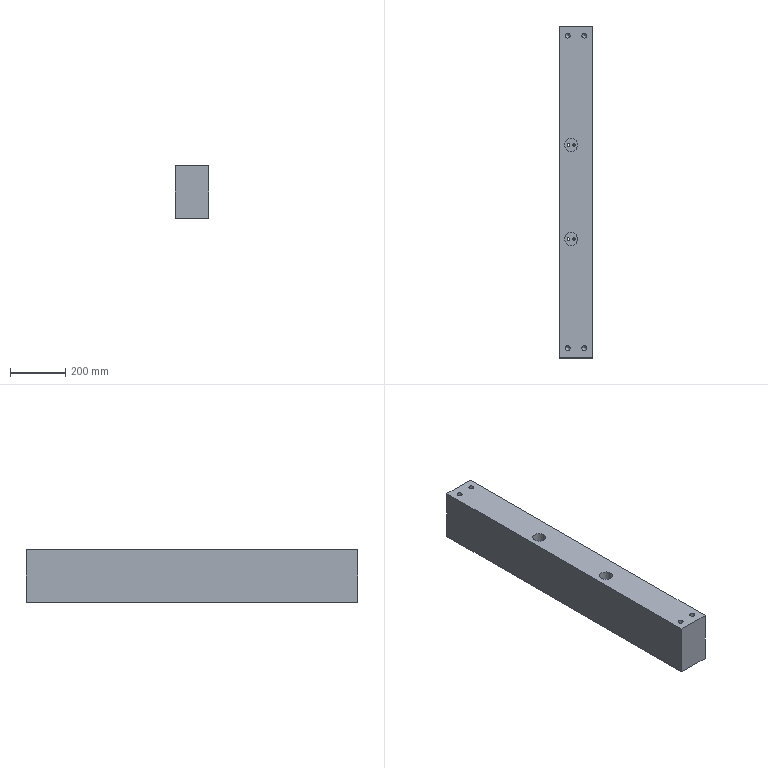Part | STEP file | lll_id4470_x_t | 1 solid | 38 faces | box 120 x 1200 x 190 mm | volume 26849134 mm3 | cylinder 18 | plane 12 | cone 8 | commonest cylinder face diameters 9 x4 14 x4 17.505 x4 17.506 x4 47 x2
STEP:
#1=CARTESIAN_POINT('',(1831.188,565.,-370.));
#2=VERTEX_POINT('',#1);
#3=CARTESIAN_POINT('',(1822.435,565.,-370.));
#4=DIRECTION('',(0.,0.,1.));
#5=DIRECTION('',(1.,0.,0.));
#6=AXIS2_PLACEMENT_3D('',#3,#4,#5);
#7=CIRCLE('',#6,8.752);
#8=EDGE_CURVE('',#2,#2,#7,.T.);
#9=ORIENTED_EDGE('',*,*,#8,.T.);
#10=EDGE_LOOP('',(#9));
#11=FACE_BOUND('',#10,.T.);
#12=CARTESIAN_POINT('',(1831.188,-565.,-370.));
#13=VERTEX_POINT('',#12);
#14=CARTESIAN_POINT('',(1822.435,-565.,-370.));
#15=DIRECTION('',(0.,0.,1.));
#16=DIRECTION('',(1.,0.,0.));
#17=AXIS2_PLACEMENT_3D('',#14,#15,#16);
#18=CIRCLE('',#17,8.752);
#19=EDGE_CURVE('',#13,#13,#18,.T.);
#20=ORIENTED_EDGE('',*,*,#19,.T.);
#21=EDGE_LOOP('',(#20));
#22=FACE_BOUND('',#21,.T.);
#23=CARTESIAN_POINT('',(1778.,-170.,-370.));
#24=VERTEX_POINT('',#23);
#25=CARTESIAN_POINT('',(1785.,-170.,-370.));
#26=DIRECTION('',(0.,0.,1.));
#27=DIRECTION('',(-1.,0.,0.));
#28=AXIS2_PLACEMENT_3D('',#25,#26,#27);
#29=CIRCLE('',#28,7.);
#30=EDGE_CURVE('',#24,#24,#29,.T.);
#31=ORIENTED_EDGE('',*,*,#30,.T.);
#32=EDGE_LOOP('',(#31));
#33=FACE_BOUND('',#32,.T.);
#34=CARTESIAN_POINT('',(1778.,170.,-370.));
#35=VERTEX_POINT('',#34);
#36=CARTESIAN_POINT('',(1785.,170.,-370.));
#37=DIRECTION('',(0.,0.,1.));
#38=DIRECTION('',(-1.,0.,0.));
#39=AXIS2_PLACEMENT_3D('',#36,#37,#38);
#40=CIRCLE('',#39,7.);
#41=EDGE_CURVE('',#35,#35,#40,.T.);
#42=ORIENTED_EDGE('',*,*,#41,.T.);
#43=EDGE_LOOP('',(#42));
#44=FACE_BOUND('',#43,.T.);
#45=CARTESIAN_POINT('',(1758.,170.,-370.));
#46=VERTEX_POINT('',#45);
#47=CARTESIAN_POINT('',(1765.,170.,-370.));
#48=DIRECTION('',(0.,0.,1.));
#49=DIRECTION('',(-1.,0.,0.));
#50=AXIS2_PLACEMENT_3D('',#47,#48,#49);
#51=CIRCLE('',#50,7.);
#52=EDGE_CURVE('',#46,#46,#51,.T.);
#53=ORIENTED_EDGE('',*,*,#52,.T.);
#54=EDGE_LOOP('',(#53));
#55=FACE_BOUND('',#54,.T.);
#56=CARTESIAN_POINT('',(1758.,-170.,-370.));
#57=VERTEX_POINT('',#56);
#58=CARTESIAN_POINT('',(1765.,-170.,-370.));
#59=DIRECTION('',(0.,0.,1.));
#60=DIRECTION('',(-1.,0.,0.));
#61=AXIS2_PLACEMENT_3D('',#58,#59,#60);
#62=CIRCLE('',#61,7.);
#63=EDGE_CURVE('',#57,#57,#62,.T.);
#64=ORIENTED_EDGE('',*,*,#63,.T.);
#65=EDGE_LOOP('',(#64));
#66=FACE_BOUND('',#65,.T.);
#67=CARTESIAN_POINT('',(1852.435,600.,-370.));
#68=VERTEX_POINT('',#67);
#69=CARTESIAN_POINT('',(1852.435,-600.,-370.));
#70=VERTEX_POINT('',#69);
#71=CARTESIAN_POINT('',(1852.435,600.,-370.));
#72=DIRECTION('',(0.,-1.,0.));
#73=VECTOR('',#72,1.);
#74=LINE('',#71,#73);
#75=EDGE_CURVE('',#68,#70,#74,.T.);
#76=ORIENTED_EDGE('',*,*,#75,.T.);
#77=CARTESIAN_POINT('',(1732.435,-600.,-370.));
#78=VERTEX_POINT('',#77);
#79=CARTESIAN_POINT('',(1852.435,-600.,-370.));
#80=DIRECTION('',(-1.,0.,0.));
#81=VECTOR('',#80,1.);
#82=LINE('',#79,#81);
#83=EDGE_CURVE('',#70,#78,#82,.T.);
#84=ORIENTED_EDGE('',*,*,#83,.T.);
#85=CARTESIAN_POINT('',(1732.435,600.,-370.));
#86=VERTEX_POINT('',#85);
#87=CARTESIAN_POINT('',(1732.435,1.,-370.));
#88=DIRECTION('',(0.,-1.,0.));
#89=VECTOR('',#88,1.);
#90=LINE('',#87,#89);
#91=EDGE_CURVE('',#86,#78,#90,.T.);
#92=ORIENTED_EDGE('',*,*,#91,.F.);
#93=CARTESIAN_POINT('',(-2117.565,600.,-370.));
#94=DIRECTION('',(1.,0.,0.));
#95=VECTOR('',#94,1.);
#96=LINE('',#93,#95);
#97=EDGE_CURVE('',#86,#68,#96,.T.);
#98=ORIENTED_EDGE('',*,*,#97,.T.);
#99=EDGE_LOOP('',(#76,#84,#92,#98));
#100=FACE_BOUND('',#99,.T.);
#101=CARTESIAN_POINT('',(1771.188,565.,-370.));
#102=VERTEX_POINT('',#101);
#103=CARTESIAN_POINT('',(1762.435,565.,-370.));
#104=DIRECTION('',(0.,0.,1.));
#105=DIRECTION('',(1.,0.,0.));
#106=AXIS2_PLACEMENT_3D('',#103,#104,#105);
#107=CIRCLE('',#106,8.752);
#108=EDGE_CURVE('',#102,#102,#107,.T.);
#109=ORIENTED_EDGE('',*,*,#108,.T.);
#110=EDGE_LOOP('',(#109));
#111=FACE_BOUND('',#110,.T.);
#112=CARTESIAN_POINT('',(1771.188,-565.,-370.));
#113=VERTEX_POINT('',#112);
#114=CARTESIAN_POINT('',(1762.435,-565.,-370.));
#115=DIRECTION('',(0.,0.,1.));
#116=DIRECTION('',(1.,0.,0.));
#117=AXIS2_PLACEMENT_3D('',#114,#115,#116);
#118=CIRCLE('',#117,8.752);
#119=EDGE_CURVE('',#113,#113,#118,.T.);
#120=ORIENTED_EDGE('',*,*,#119,.T.);
#121=EDGE_LOOP('',(#120));
#122=FACE_BOUND('',#121,.T.);
#123=CARTESIAN_POINT('',(4038.751,1.,-370.));
#124=DIRECTION('',(0.,0.,-1.));
#125=DIRECTION('',(-1.,0.,0.));
#126=AXIS2_PLACEMENT_3D('',#123,#124,#125);
#127=PLANE('',#126);
#128=ADVANCED_FACE('',(#11,#22,#33,#44,#55,#66,#100,#111,#122),#127,.T.);
#129=CARTESIAN_POINT('',(1852.435,600.,-180.));
#130=VERTEX_POINT('',#129);
#131=CARTESIAN_POINT('',(1852.435,-600.,-180.));
#132=VERTEX_POINT('',#131);
#133=CARTESIAN_POINT('',(1852.435,1.,-180.));
#134=DIRECTION('',(0.,-1.,0.));
#135=VECTOR('',#134,1.);
#136=LINE('',#133,#135);
#137=EDGE_CURVE('',#130,#132,#136,.T.);
#138=ORIENTED_EDGE('',*,*,#137,.T.);
#139=CARTESIAN_POINT('',(1852.435,-600.,-182.5));
#140=DIRECTION('',(0.,0.,-1.));
#141=VECTOR('',#140,1.);
#142=LINE('',#139,#141);
#143=EDGE_CURVE('',#132,#70,#142,.T.);
#144=ORIENTED_EDGE('',*,*,#143,.T.);
#145=ORIENTED_EDGE('',*,*,#75,.F.);
#146=CARTESIAN_POINT('',(1852.435,600.,-182.5));
#147=DIRECTION('',(0.,0.,-1.));
#148=VECTOR('',#147,1.);
#149=LINE('',#146,#148);
#150=EDGE_CURVE('',#130,#68,#149,.T.);
#151=ORIENTED_EDGE('',*,*,#150,.F.);
#152=EDGE_LOOP('',(#138,#144,#145,#151));
#153=FACE_OUTER_BOUND('',#152,.T.);
#154=CARTESIAN_POINT('',(1852.435,600.,-182.5));
#155=DIRECTION('',(1.,0.,0.));
#156=DIRECTION('',(0.,0.,-1.));
#157=AXIS2_PLACEMENT_3D('',#154,#155,#156);
#158=PLANE('',#157);
#159=ADVANCED_FACE('',(#153),#158,.T.);
#160=CARTESIAN_POINT('',(1753.682,565.,-180.));
#161=VERTEX_POINT('',#160);
#162=CARTESIAN_POINT('',(1762.435,565.,-180.));
#163=DIRECTION('',(0.,0.,-1.));
#164=DIRECTION('',(-1.,0.,0.));
#165=AXIS2_PLACEMENT_3D('',#162,#163,#164);
#166=CIRCLE('',#165,8.753);
#167=EDGE_CURVE('',#161,#161,#166,.T.);
#168=ORIENTED_EDGE('',*,*,#167,.T.);
#169=EDGE_LOOP('',(#168));
#170=FACE_BOUND('',#169,.T.);
#171=CARTESIAN_POINT('',(1753.682,-565.,-180.));
#172=VERTEX_POINT('',#171);
#173=CARTESIAN_POINT('',(1762.435,-565.,-180.));
#174=DIRECTION('',(0.,0.,-1.));
#175=DIRECTION('',(-1.,0.,0.));
#176=AXIS2_PLACEMENT_3D('',#173,#174,#175);
#177=CIRCLE('',#176,8.753);
#178=EDGE_CURVE('',#172,#172,#177,.T.);
#179=ORIENTED_EDGE('',*,*,#178,.T.);
#180=EDGE_LOOP('',(#179));
#181=FACE_BOUND('',#180,.T.);
#182=CARTESIAN_POINT('',(1813.682,-565.,-180.));
#183=VERTEX_POINT('',#182);
#184=CARTESIAN_POINT('',(1822.435,-565.,-180.));
#185=DIRECTION('',(0.,0.,-1.));
#186=DIRECTION('',(-1.,0.,0.));
#187=AXIS2_PLACEMENT_3D('',#184,#185,#186);
#188=CIRCLE('',#187,8.753);
#189=EDGE_CURVE('',#183,#183,#188,.T.);
#190=ORIENTED_EDGE('',*,*,#189,.T.);
#191=EDGE_LOOP('',(#190));
#192=FACE_BOUND('',#191,.T.);
#193=CARTESIAN_POINT('',(1813.682,565.,-180.));
#194=VERTEX_POINT('',#193);
#195=CARTESIAN_POINT('',(1822.435,565.,-180.));
#196=DIRECTION('',(0.,0.,-1.));
#197=DIRECTION('',(-1.,0.,0.));
#198=AXIS2_PLACEMENT_3D('',#195,#196,#197);
#199=CIRCLE('',#198,8.753);
#200=EDGE_CURVE('',#194,#194,#199,.T.);
#201=ORIENTED_EDGE('',*,*,#200,.T.);
#202=EDGE_LOOP('',(#201));
#203=FACE_BOUND('',#202,.T.);
#204=CARTESIAN_POINT('',(1732.435,-600.,-180.));
#205=VERTEX_POINT('',#204);
#206=CARTESIAN_POINT('',(4038.751,-600.,-180.));
#207=DIRECTION('',(-1.,0.,0.));
#208=VECTOR('',#207,1.);
#209=LINE('',#206,#208);
#210=EDGE_CURVE('',#132,#205,#209,.T.);
#211=ORIENTED_EDGE('',*,*,#210,.F.);
#212=ORIENTED_EDGE('',*,*,#137,.F.);
#213=CARTESIAN_POINT('',(1732.435,600.,-180.));
#214=VERTEX_POINT('',#213);
#215=CARTESIAN_POINT('',(4038.751,600.,-180.));
#216=DIRECTION('',(1.,0.,0.));
#217=VECTOR('',#216,1.);
#218=LINE('',#215,#217);
#219=EDGE_CURVE('',#214,#130,#218,.T.);
#220=ORIENTED_EDGE('',*,*,#219,.F.);
#221=CARTESIAN_POINT('',(1732.435,0.,-180.));
#222=DIRECTION('',(0.,1.,0.));
#223=VECTOR('',#222,1.);
#224=LINE('',#221,#223);
#225=EDGE_CURVE('',#205,#214,#224,.T.);
#226=ORIENTED_EDGE('',*,*,#225,.F.);
#227=EDGE_LOOP('',(#211,#212,#220,#226));
#228=FACE_BOUND('',#227,.T.);
#229=CARTESIAN_POINT('',(1751.5,170.,-180.));
#230=VERTEX_POINT('',#229);
#231=CARTESIAN_POINT('',(1775.,170.,-180.));
#232=DIRECTION('',(0.,0.,-1.));
#233=DIRECTION('',(-1.,0.,0.));
#234=AXIS2_PLACEMENT_3D('',#231,#232,#233);
#235=CIRCLE('',#234,23.5);
#236=EDGE_CURVE('',#230,#230,#235,.T.);
#237=ORIENTED_EDGE('',*,*,#236,.T.);
#238=EDGE_LOOP('',(#237));
#239=FACE_BOUND('',#238,.T.);
#240=CARTESIAN_POINT('',(1751.5,-170.,-180.));
#241=VERTEX_POINT('',#240);
#242=CARTESIAN_POINT('',(1775.,-170.,-180.));
#243=DIRECTION('',(0.,0.,-1.));
#244=DIRECTION('',(-1.,0.,0.));
#245=AXIS2_PLACEMENT_3D('',#242,#243,#244);
#246=CIRCLE('',#245,23.5);
#247=EDGE_CURVE('',#241,#241,#246,.T.);
#248=ORIENTED_EDGE('',*,*,#247,.T.);
#249=EDGE_LOOP('',(#248));
#250=FACE_BOUND('',#249,.T.);
#251=CARTESIAN_POINT('',(4038.751,1.,-180.));
#252=DIRECTION('',(0.,0.,-1.));
#253=DIRECTION('',(-1.,0.,0.));
#254=AXIS2_PLACEMENT_3D('',#251,#252,#253);
#255=PLANE('',#254);
#256=ADVANCED_FACE('',(#170,#181,#192,#203,#228,#239,#250),#255,.F.);
#257=ORIENTED_EDGE('',*,*,#91,.T.);
#258=CARTESIAN_POINT('',(1732.435,-600.,-251.25));
#259=DIRECTION('',(0.,0.,-1.));
#260=VECTOR('',#259,1.);
#261=LINE('',#258,#260);
#262=EDGE_CURVE('',#205,#78,#261,.T.);
#263=ORIENTED_EDGE('',*,*,#262,.F.);
#264=ORIENTED_EDGE('',*,*,#225,.T.);
#265=CARTESIAN_POINT('',(1732.435,600.,-251.25));
#266=DIRECTION('',(0.,0.,1.));
#267=VECTOR('',#266,1.);
#268=LINE('',#265,#267);
#269=EDGE_CURVE('',#86,#214,#268,.T.);
#270=ORIENTED_EDGE('',*,*,#269,.F.);
#271=EDGE_LOOP('',(#257,#263,#264,#270));
#272=FACE_OUTER_BOUND('',#271,.T.);
#273=CARTESIAN_POINT('',(1732.435,0.,-251.25));
#274=DIRECTION('',(1.,0.,0.));
#275=DIRECTION('',(0.,0.,-1.));
#276=AXIS2_PLACEMENT_3D('',#273,#274,#275);
#277=PLANE('',#276);
#278=ADVANCED_FACE('',(#272),#277,.F.);
#279=ORIENTED_EDGE('',*,*,#262,.T.);
#280=ORIENTED_EDGE('',*,*,#83,.F.);
#281=ORIENTED_EDGE('',*,*,#143,.F.);
#282=ORIENTED_EDGE('',*,*,#210,.T.);
#283=EDGE_LOOP('',(#279,#280,#281,#282));
#284=FACE_OUTER_BOUND('',#283,.T.);
#285=CARTESIAN_POINT('',(1852.435,-600.,-182.5));
#286=DIRECTION('',(0.,-1.,0.));
#287=DIRECTION('',(0.,0.,-1.));
#288=AXIS2_PLACEMENT_3D('',#285,#286,#287);
#289=PLANE('',#288);
#290=ADVANCED_FACE('',(#284),#289,.T.);
#291=ORIENTED_EDGE('',*,*,#269,.T.);
#292=ORIENTED_EDGE('',*,*,#219,.T.);
#293=ORIENTED_EDGE('',*,*,#150,.T.);
#294=ORIENTED_EDGE('',*,*,#97,.F.);
#295=EDGE_LOOP('',(#291,#292,#293,#294));
#296=FACE_OUTER_BOUND('',#295,.T.);
#297=CARTESIAN_POINT('',(-2117.565,600.,-182.5));
#298=DIRECTION('',(0.,1.,0.));
#299=DIRECTION('',(0.,0.,1.));
#300=AXIS2_PLACEMENT_3D('',#297,#298,#299);
#301=PLANE('',#300);
#302=ADVANCED_FACE('',(#296),#301,.T.);
#303=CARTESIAN_POINT('',(1780.5,170.,-322.));
#304=VERTEX_POINT('',#303);
#305=CARTESIAN_POINT('',(1785.,170.,-322.));
#306=DIRECTION('',(0.,0.,-1.));
#307=DIRECTION('',(-1.,0.,0.));
#308=AXIS2_PLACEMENT_3D('',#305,#306,#307);
#309=CIRCLE('',#308,4.5);
#310=EDGE_CURVE('',#304,#304,#309,.T.);
#311=ORIENTED_EDGE('',*,*,#310,.F.);
#312=EDGE_LOOP('',(#311));
#313=FACE_BOUND('',#312,.T.);
#314=CARTESIAN_POINT('',(1778.,170.,-322.));
#315=VERTEX_POINT('',#314);
#316=CARTESIAN_POINT('',(1785.,170.,-322.));
#317=DIRECTION('',(0.,0.,1.));
#318=DIRECTION('',(-1.,0.,0.));
#319=AXIS2_PLACEMENT_3D('',#316,#317,#318);
#320=CIRCLE('',#319,7.);
#321=EDGE_CURVE('',#315,#315,#320,.T.);
#322=ORIENTED_EDGE('',*,*,#321,.F.);
#323=EDGE_LOOP('',(#322));
#324=FACE_BOUND('',#323,.T.);
#325=CARTESIAN_POINT('',(1785.,170.,-322.));
#326=DIRECTION('',(0.,0.,-1.));
#327=DIRECTION('',(-1.,0.,0.));
#328=AXIS2_PLACEMENT_3D('',#325,#326,#327);
#329=PLANE('',#328);
#330=ADVANCED_FACE('',(#313,#324),#329,.T.);
#331=ORIENTED_EDGE('',*,*,#41,.F.);
#332=EDGE_LOOP('',(#331));
#333=FACE_BOUND('',#332,.T.);
#334=ORIENTED_EDGE('',*,*,#321,.T.);
#335=EDGE_LOOP('',(#334));
#336=FACE_BOUND('',#335,.T.);
#337=CARTESIAN_POINT('',(1785.,170.,-432.));
#338=DIRECTION('',(0.,0.,1.));
#339=DIRECTION('',(1.,0.,0.));
#340=AXIS2_PLACEMENT_3D('',#337,#338,#339);
#341=CYLINDRICAL_SURFACE('',#340,7.);
#342=ADVANCED_FACE('',(#333,#336),#341,.F.);
#343=ORIENTED_EDGE('',*,*,#52,.F.);
#344=EDGE_LOOP('',(#343));
#345=FACE_BOUND('',#344,.T.);
#346=CARTESIAN_POINT('',(1758.,170.,-322.));
#347=VERTEX_POINT('',#346);
#348=CARTESIAN_POINT('',(1765.,170.,-322.));
#349=DIRECTION('',(0.,0.,1.));
#350=DIRECTION('',(-1.,0.,0.));
#351=AXIS2_PLACEMENT_3D('',#348,#349,#350);
#352=CIRCLE('',#351,7.);
#353=EDGE_CURVE('',#347,#347,#352,.T.);
#354=ORIENTED_EDGE('',*,*,#353,.T.);
#355=EDGE_LOOP('',(#354));
#356=FACE_BOUND('',#355,.T.);
#357=CARTESIAN_POINT('',(1765.,170.,-432.));
#358=DIRECTION('',(0.,0.,1.));
#359=DIRECTION('',(1.,0.,0.));
#360=AXIS2_PLACEMENT_3D('',#357,#358,#359);
#361=CYLINDRICAL_SURFACE('',#360,7.);
#362=ADVANCED_FACE('',(#345,#356),#361,.F.);
#363=ORIENTED_EDGE('',*,*,#353,.F.);
#364=EDGE_LOOP('',(#363));
#365=FACE_BOUND('',#364,.T.);
#366=CARTESIAN_POINT('',(1760.5,170.,-322.));
#367=VERTEX_POINT('',#366);
#368=CARTESIAN_POINT('',(1765.,170.,-322.));
#369=DIRECTION('',(0.,0.,1.));
#370=DIRECTION('',(-1.,0.,0.));
#371=AXIS2_PLACEMENT_3D('',#368,#369,#370);
#372=CIRCLE('',#371,4.5);
#373=EDGE_CURVE('',#367,#367,#372,.T.);
#374=ORIENTED_EDGE('',*,*,#373,.T.);
#375=EDGE_LOOP('',(#374));
#376=FACE_BOUND('',#375,.T.);
#377=CARTESIAN_POINT('',(1765.,170.,-322.));
#378=DIRECTION('',(0.,0.,-1.));
#379=DIRECTION('',(-1.,0.,0.));
#380=AXIS2_PLACEMENT_3D('',#377,#378,#379);
#381=PLANE('',#380);
#382=ADVANCED_FACE('',(#365,#376),#381,.T.);
#383=CARTESIAN_POINT('',(1760.5,170.,-292.));
#384=VERTEX_POINT('',#383);
#385=CARTESIAN_POINT('',(1765.,170.,-292.));
#386=DIRECTION('',(0.,0.,1.));
#387=DIRECTION('',(-1.,0.,0.));
#388=AXIS2_PLACEMENT_3D('',#385,#386,#387);
#389=CIRCLE('',#388,4.5);
#390=EDGE_CURVE('',#384,#384,#389,.T.);
#391=ORIENTED_EDGE('',*,*,#390,.T.);
#392=EDGE_LOOP('',(#391));
#393=FACE_BOUND('',#392,.T.);
#394=ORIENTED_EDGE('',*,*,#373,.F.);
#395=EDGE_LOOP('',(#394));
#396=FACE_BOUND('',#395,.T.);
#397=CARTESIAN_POINT('',(1765.,170.,-432.));
#398=DIRECTION('',(0.,0.,1.));
#399=DIRECTION('',(1.,0.,0.));
#400=AXIS2_PLACEMENT_3D('',#397,#398,#399);
#401=CYLINDRICAL_SURFACE('',#400,4.5);
#402=ADVANCED_FACE('',(#393,#396),#401,.F.);
#403=CARTESIAN_POINT('',(1751.5,170.,-292.));
#404=VERTEX_POINT('',#403);
#405=CARTESIAN_POINT('',(1775.,170.,-292.));
#406=DIRECTION('',(0.,0.,-1.));
#407=DIRECTION('',(-1.,0.,0.));
#408=AXIS2_PLACEMENT_3D('',#405,#406,#407);
#409=CIRCLE('',#408,23.5);
#410=EDGE_CURVE('',#404,#404,#409,.T.);
#411=ORIENTED_EDGE('',*,*,#410,.T.);
#412=EDGE_LOOP('',(#411));
#413=FACE_BOUND('',#412,.T.);
#414=ORIENTED_EDGE('',*,*,#236,.F.);
#415=EDGE_LOOP('',(#414));
#416=FACE_BOUND('',#415,.T.);
#417=CARTESIAN_POINT('',(1775.,170.,-288.));
#418=DIRECTION('',(0.,0.,1.));
#419=DIRECTION('',(1.,0.,0.));
#420=AXIS2_PLACEMENT_3D('',#417,#418,#419);
#421=CYLINDRICAL_SURFACE('',#420,23.5);
#422=ADVANCED_FACE('',(#413,#416),#421,.F.);
#423=CARTESIAN_POINT('',(1780.5,170.,-292.));
#424=VERTEX_POINT('',#423);
#425=CARTESIAN_POINT('',(1785.,170.,-292.));
#426=DIRECTION('',(0.,0.,-1.));
#427=DIRECTION('',(-1.,0.,0.));
#428=AXIS2_PLACEMENT_3D('',#425,#426,#427);
#429=CIRCLE('',#428,4.5);
#430=EDGE_CURVE('',#424,#424,#429,.T.);
#431=ORIENTED_EDGE('',*,*,#430,.F.);
#432=EDGE_LOOP('',(#431));
#433=FACE_BOUND('',#432,.T.);
#434=ORIENTED_EDGE('',*,*,#310,.T.);
#435=EDGE_LOOP('',(#434));
#436=FACE_BOUND('',#435,.T.);
#437=CARTESIAN_POINT('',(1785.,170.,-432.));
#438=DIRECTION('',(0.,0.,1.));
#439=DIRECTION('',(1.,0.,0.));
#440=AXIS2_PLACEMENT_3D('',#437,#438,#439);
#441=CYLINDRICAL_SURFACE('',#440,4.5);
#442=ADVANCED_FACE('',(#433,#436),#441,.F.);
#443=ORIENTED_EDGE('',*,*,#410,.F.);
#444=EDGE_LOOP('',(#443));
#445=FACE_BOUND('',#444,.T.);
#446=ORIENTED_EDGE('',*,*,#390,.F.);
#447=EDGE_LOOP('',(#446));
#448=FACE_BOUND('',#447,.T.);
#449=ORIENTED_EDGE('',*,*,#430,.T.);
#450=EDGE_LOOP('',(#449));
#451=FACE_BOUND('',#450,.T.);
#452=CARTESIAN_POINT('',(1785.8,170.,-292.));
#453=DIRECTION('',(0.,0.,-1.));
#454=DIRECTION('',(1.,0.,0.));
#455=AXIS2_PLACEMENT_3D('',#452,#453,#454);
#456=PLANE('',#455);
#457=ADVANCED_FACE('',(#445,#448,#451),#456,.F.);
#458=CARTESIAN_POINT('',(1780.5,-170.,-322.));
#459=VERTEX_POINT('',#458);
#460=CARTESIAN_POINT('',(1785.,-170.,-322.));
#461=DIRECTION('',(0.,0.,-1.));
#462=DIRECTION('',(-1.,0.,0.));
#463=AXIS2_PLACEMENT_3D('',#460,#461,#462);
#464=CIRCLE('',#463,4.5);
#465=EDGE_CURVE('',#459,#459,#464,.T.);
#466=ORIENTED_EDGE('',*,*,#465,.F.);
#467=EDGE_LOOP('',(#466));
#468=FACE_BOUND('',#467,.T.);
#469=CARTESIAN_POINT('',(1778.,-170.,-322.));
#470=VERTEX_POINT('',#469);
#471=CARTESIAN_POINT('',(1785.,-170.,-322.));
#472=DIRECTION('',(0.,0.,1.));
#473=DIRECTION('',(-1.,0.,0.));
#474=AXIS2_PLACEMENT_3D('',#471,#472,#473);
#475=CIRCLE('',#474,7.);
#476=EDGE_CURVE('',#470,#470,#475,.T.);
#477=ORIENTED_EDGE('',*,*,#476,.F.);
#478=EDGE_LOOP('',(#477));
#479=FACE_BOUND('',#478,.T.);
#480=CARTESIAN_POINT('',(1785.,-170.,-322.));
#481=DIRECTION('',(0.,0.,-1.));
#482=DIRECTION('',(-1.,0.,0.));
#483=AXIS2_PLACEMENT_3D('',#480,#481,#482);
#484=PLANE('',#483);
#485=ADVANCED_FACE('',(#468,#479),#484,.T.);
#486=ORIENTED_EDGE('',*,*,#30,.F.);
#487=EDGE_LOOP('',(#486));
#488=FACE_BOUND('',#487,.T.);
#489=ORIENTED_EDGE('',*,*,#476,.T.);
#490=EDGE_LOOP('',(#489));
#491=FACE_BOUND('',#490,.T.);
#492=CARTESIAN_POINT('',(1785.,-170.,-432.));
#493=DIRECTION('',(0.,0.,1.));
#494=DIRECTION('',(1.,0.,0.));
#495=AXIS2_PLACEMENT_3D('',#492,#493,#494);
#496=CYLINDRICAL_SURFACE('',#495,7.);
#497=ADVANCED_FACE('',(#488,#491),#496,.F.);
#498=ORIENTED_EDGE('',*,*,#63,.F.);
#499=EDGE_LOOP('',(#498));
#500=FACE_BOUND('',#499,.T.);
#501=CARTESIAN_POINT('',(1758.,-170.,-322.));
#502=VERTEX_POINT('',#501);
#503=CARTESIAN_POINT('',(1765.,-170.,-322.));
#504=DIRECTION('',(0.,0.,1.));
#505=DIRECTION('',(-1.,0.,0.));
#506=AXIS2_PLACEMENT_3D('',#503,#504,#505);
#507=CIRCLE('',#506,7.);
#508=EDGE_CURVE('',#502,#502,#507,.T.);
#509=ORIENTED_EDGE('',*,*,#508,.T.);
#510=EDGE_LOOP('',(#509));
#511=FACE_BOUND('',#510,.T.);
#512=CARTESIAN_POINT('',(1765.,-170.,-432.));
#513=DIRECTION('',(0.,0.,1.));
#514=DIRECTION('',(1.,0.,0.));
#515=AXIS2_PLACEMENT_3D('',#512,#513,#514);
#516=CYLINDRICAL_SURFACE('',#515,7.);
#517=ADVANCED_FACE('',(#500,#511),#516,.F.);
#518=ORIENTED_EDGE('',*,*,#508,.F.);
#519=EDGE_LOOP('',(#518));
#520=FACE_BOUND('',#519,.T.);
#521=CARTESIAN_POINT('',(1760.5,-170.,-322.));
#522=VERTEX_POINT('',#521);
#523=CARTESIAN_POINT('',(1765.,-170.,-322.));
#524=DIRECTION('',(0.,0.,1.));
#525=DIRECTION('',(-1.,0.,0.));
#526=AXIS2_PLACEMENT_3D('',#523,#524,#525);
#527=CIRCLE('',#526,4.5);
#528=EDGE_CURVE('',#522,#522,#527,.T.);
#529=ORIENTED_EDGE('',*,*,#528,.T.);
#530=EDGE_LOOP('',(#529));
#531=FACE_BOUND('',#530,.T.);
#532=CARTESIAN_POINT('',(1765.,-170.,-322.));
#533=DIRECTION('',(0.,0.,-1.));
#534=DIRECTION('',(-1.,0.,0.));
#535=AXIS2_PLACEMENT_3D('',#532,#533,#534);
#536=PLANE('',#535);
#537=ADVANCED_FACE('',(#520,#531),#536,.T.);
#538=CARTESIAN_POINT('',(1760.5,-170.,-292.));
#539=VERTEX_POINT('',#538);
#540=CARTESIAN_POINT('',(1765.,-170.,-292.));
#541=DIRECTION('',(0.,0.,1.));
#542=DIRECTION('',(-1.,0.,0.));
#543=AXIS2_PLACEMENT_3D('',#540,#541,#542);
#544=CIRCLE('',#543,4.5);
#545=EDGE_CURVE('',#539,#539,#544,.T.);
#546=ORIENTED_EDGE('',*,*,#545,.T.);
#547=EDGE_LOOP('',(#546));
#548=FACE_BOUND('',#547,.T.);
#549=ORIENTED_EDGE('',*,*,#528,.F.);
#550=EDGE_LOOP('',(#549));
#551=FACE_BOUND('',#550,.T.);
#552=CARTESIAN_POINT('',(1765.,-170.,-432.));
#553=DIRECTION('',(0.,0.,1.));
#554=DIRECTION('',(1.,0.,0.));
#555=AXIS2_PLACEMENT_3D('',#552,#553,#554);
#556=CYLINDRICAL_SURFACE('',#555,4.5);
#557=ADVANCED_FACE('',(#548,#551),#556,.F.);
#558=CARTESIAN_POINT('',(1751.5,-170.,-292.));
#559=VERTEX_POINT('',#558);
#560=CARTESIAN_POINT('',(1775.,-170.,-292.));
#561=DIRECTION('',(0.,0.,-1.));
#562=DIRECTION('',(-1.,0.,0.));
#563=AXIS2_PLACEMENT_3D('',#560,#561,#562);
#564=CIRCLE('',#563,23.5);
#565=EDGE_CURVE('',#559,#559,#564,.T.);
#566=ORIENTED_EDGE('',*,*,#565,.T.);
#567=EDGE_LOOP('',(#566));
#568=FACE_BOUND('',#567,.T.);
#569=ORIENTED_EDGE('',*,*,#247,.F.);
#570=EDGE_LOOP('',(#569));
#571=FACE_BOUND('',#570,.T.);
#572=CARTESIAN_POINT('',(1775.,-170.,-288.));
#573=DIRECTION('',(0.,0.,1.));
#574=DIRECTION('',(1.,0.,0.));
#575=AXIS2_PLACEMENT_3D('',#572,#573,#574);
#576=CYLINDRICAL_SURFACE('',#575,23.5);
#577=ADVANCED_FACE('',(#568,#571),#576,.F.);
#578=CARTESIAN_POINT('',(1780.5,-170.,-292.));
#579=VERTEX_POINT('',#578);
#580=CARTESIAN_POINT('',(1785.,-170.,-292.));
#581=DIRECTION('',(0.,0.,-1.));
#582=DIRECTION('',(-1.,0.,0.));
#583=AXIS2_PLACEMENT_3D('',#580,#581,#582);
#584=CIRCLE('',#583,4.5);
#585=EDGE_CURVE('',#579,#579,#584,.T.);
#586=ORIENTED_EDGE('',*,*,#585,.F.);
#587=EDGE_LOOP('',(#586));
#588=FACE_BOUND('',#587,.T.);
#589=ORIENTED_EDGE('',*,*,#465,.T.);
#590=EDGE_LOOP('',(#589));
#591=FACE_BOUND('',#590,.T.);
#592=CARTESIAN_POINT('',(1785.,-170.,-432.));
#593=DIRECTION('',(0.,0.,1.));
#594=DIRECTION('',(1.,0.,0.));
#595=AXIS2_PLACEMENT_3D('',#592,#593,#594);
#596=CYLINDRICAL_SURFACE('',#595,4.5);
#597=ADVANCED_FACE('',(#588,#591),#596,.F.);
#598=ORIENTED_EDGE('',*,*,#565,.F.);
#599=EDGE_LOOP('',(#598));
#600=FACE_BOUND('',#599,.T.);
#601=ORIENTED_EDGE('',*,*,#545,.F.);
#602=EDGE_LOOP('',(#601));
#603=FACE_BOUND('',#602,.T.);
#604=ORIENTED_EDGE('',*,*,#585,.T.);
#605=EDGE_LOOP('',(#604));
#606=FACE_BOUND('',#605,.T.);
#607=CARTESIAN_POINT('',(1785.8,-170.,-292.));
#608=DIRECTION('',(0.,0.,-1.));
#609=DIRECTION('',(1.,0.,0.));
#610=AXIS2_PLACEMENT_3D('',#607,#608,#609);
#611=PLANE('',#610);
#612=ADVANCED_FACE('',(#600,#603,#606),#611,.F.);
#613=CARTESIAN_POINT('',(1831.188,-565.,-328.747));
#614=VERTEX_POINT('',#613);
#615=CARTESIAN_POINT('',(1822.435,-565.,-328.747));
#616=DIRECTION('',(0.,0.,1.));
#617=DIRECTION('',(1.,0.,0.));
#618=AXIS2_PLACEMENT_3D('',#615,#616,#617);
#619=CIRCLE('',#618,8.752);
#620=EDGE_CURVE('',#614,#614,#619,.T.);
#621=ORIENTED_EDGE('',*,*,#620,.T.);
#622=EDGE_LOOP('',(#621));
#623=FACE_BOUND('',#622,.T.);
#624=ORIENTED_EDGE('',*,*,#19,.F.);
#625=EDGE_LOOP('',(#624));
#626=FACE_BOUND('',#625,.T.);
#627=CARTESIAN_POINT('',(1822.435,-565.,-370.));
#628=DIRECTION('',(0.,0.,1.));
#629=DIRECTION('',(-1.,0.,0.));
#630=AXIS2_PLACEMENT_3D('',#627,#628,#629);
#631=CYLINDRICAL_SURFACE('',#630,8.752);
#632=ADVANCED_FACE('',(#623,#626),#631,.F.);
#633=CARTESIAN_POINT('',(1822.435,-565.,-319.994));
#634=VERTEX_POINT('',#633);
#635=VERTEX_LOOP('',#634);
#636=FACE_BOUND('',#635,.T.);
#637=ORIENTED_EDGE('',*,*,#620,.F.);
#638=EDGE_LOOP('',(#637));
#639=FACE_BOUND('',#638,.T.);
#640=CARTESIAN_POINT('',(1822.435,-565.,-328.747));
#641=DIRECTION('',(0.,0.,-1.));
#642=DIRECTION('',(1.,0.,0.));
#643=AXIS2_PLACEMENT_3D('',#640,#641,#642);
#644=CONICAL_SURFACE('',#643,8.752,45.);
#645=ADVANCED_FACE('',(#636,#639),#644,.F.);
#646=CARTESIAN_POINT('',(1771.188,565.,-328.747));
#647=VERTEX_POINT('',#646);
#648=CARTESIAN_POINT('',(1762.435,565.,-328.747));
#649=DIRECTION('',(0.,0.,1.));
#650=DIRECTION('',(1.,0.,0.));
#651=AXIS2_PLACEMENT_3D('',#648,#649,#650);
#652=CIRCLE('',#651,8.752);
#653=EDGE_CURVE('',#647,#647,#652,.T.);
#654=ORIENTED_EDGE('',*,*,#653,.T.);
#655=EDGE_LOOP('',(#654));
#656=FACE_BOUND('',#655,.T.);
#657=ORIENTED_EDGE('',*,*,#108,.F.);
#658=EDGE_LOOP('',(#657));
#659=FACE_BOUND('',#658,.T.);
#660=CARTESIAN_POINT('',(1762.435,565.,-370.));
#661=DIRECTION('',(0.,0.,1.));
#662=DIRECTION('',(-1.,0.,0.));
#663=AXIS2_PLACEMENT_3D('',#660,#661,#662);
#664=CYLINDRICAL_SURFACE('',#663,8.752);
#665=ADVANCED_FACE('',(#656,#659),#664,.F.);
#666=CARTESIAN_POINT('',(1762.435,565.,-319.994));
#667=VERTEX_POINT('',#666);
#668=VERTEX_LOOP('',#667);
#669=FACE_BOUND('',#668,.T.);
#670=ORIENTED_EDGE('',*,*,#653,.F.);
#671=EDGE_LOOP('',(#670));
#672=FACE_BOUND('',#671,.T.);
#673=CARTESIAN_POINT('',(1762.435,565.,-328.747));
#674=DIRECTION('',(0.,0.,-1.));
#675=DIRECTION('',(1.,0.,0.));
#676=AXIS2_PLACEMENT_3D('',#673,#674,#675);
#677=CONICAL_SURFACE('',#676,8.752,45.);
#678=ADVANCED_FACE('',(#669,#672),#677,.F.);
#679=CARTESIAN_POINT('',(1831.188,565.,-328.747));
#680=VERTEX_POINT('',#679);
#681=CARTESIAN_POINT('',(1822.435,565.,-328.747));
#682=DIRECTION('',(0.,0.,1.));
#683=DIRECTION('',(1.,0.,0.));
#684=AXIS2_PLACEMENT_3D('',#681,#682,#683);
#685=CIRCLE('',#684,8.752);
#686=EDGE_CURVE('',#680,#680,#685,.T.);
#687=ORIENTED_EDGE('',*,*,#686,.T.);
#688=EDGE_LOOP('',(#687));
#689=FACE_BOUND('',#688,.T.);
#690=ORIENTED_EDGE('',*,*,#8,.F.);
#691=EDGE_LOOP('',(#690));
#692=FACE_BOUND('',#691,.T.);
#693=CARTESIAN_POINT('',(1822.435,565.,-370.));
#694=DIRECTION('',(0.,0.,1.));
#695=DIRECTION('',(-1.,0.,0.));
#696=AXIS2_PLACEMENT_3D('',#693,#694,#695);
#697=CYLINDRICAL_SURFACE('',#696,8.752);
#698=ADVANCED_FACE('',(#689,#692),#697,.F.);
#699=CARTESIAN_POINT('',(1822.435,565.,-319.994));
#700=VERTEX_POINT('',#699);
#701=VERTEX_LOOP('',#700);
#702=FACE_BOUND('',#701,.T.);
#703=ORIENTED_EDGE('',*,*,#686,.F.);
#704=EDGE_LOOP('',(#703));
#705=FACE_BOUND('',#704,.T.);
#706=CARTESIAN_POINT('',(1822.435,565.,-328.747));
#707=DIRECTION('',(0.,0.,-1.));
#708=DIRECTION('',(1.,0.,0.));
#709=AXIS2_PLACEMENT_3D('',#706,#707,#708);
#710=CONICAL_SURFACE('',#709,8.752,45.);
#711=ADVANCED_FACE('',(#702,#705),#710,.F.);
#712=CARTESIAN_POINT('',(1771.188,-565.,-328.747));
#713=VERTEX_POINT('',#712);
#714=CARTESIAN_POINT('',(1762.435,-565.,-328.747));
#715=DIRECTION('',(0.,0.,1.));
#716=DIRECTION('',(1.,0.,0.));
#717=AXIS2_PLACEMENT_3D('',#714,#715,#716);
#718=CIRCLE('',#717,8.752);
#719=EDGE_CURVE('',#713,#713,#718,.T.);
#720=ORIENTED_EDGE('',*,*,#719,.T.);
#721=EDGE_LOOP('',(#720));
#722=FACE_BOUND('',#721,.T.);
#723=ORIENTED_EDGE('',*,*,#119,.F.);
#724=EDGE_LOOP('',(#723));
#725=FACE_BOUND('',#724,.T.);
#726=CARTESIAN_POINT('',(1762.435,-565.,-370.));
#727=DIRECTION('',(0.,0.,1.));
#728=DIRECTION('',(-1.,0.,0.));
#729=AXIS2_PLACEMENT_3D('',#726,#727,#728);
#730=CYLINDRICAL_SURFACE('',#729,8.752);
#731=ADVANCED_FACE('',(#722,#725),#730,.F.);
#732=CARTESIAN_POINT('',(1762.435,-565.,-319.994));
#733=VERTEX_POINT('',#732);
#734=VERTEX_LOOP('',#733);
#735=FACE_BOUND('',#734,.T.);
#736=ORIENTED_EDGE('',*,*,#719,.F.);
#737=EDGE_LOOP('',(#736));
#738=FACE_BOUND('',#737,.T.);
#739=CARTESIAN_POINT('',(1762.435,-565.,-328.747));
#740=DIRECTION('',(0.,0.,-1.));
#741=DIRECTION('',(1.,0.,0.));
#742=AXIS2_PLACEMENT_3D('',#739,#740,#741);
#743=CONICAL_SURFACE('',#742,8.752,45.);
#744=ADVANCED_FACE('',(#735,#738),#743,.F.);
#745=CARTESIAN_POINT('',(1813.682,565.,-221.253));
#746=VERTEX_POINT('',#745);
#747=CARTESIAN_POINT('',(1822.435,565.,-221.253));
#748=DIRECTION('',(0.,0.,-1.));
#749=DIRECTION('',(-1.,0.,0.));
#750=AXIS2_PLACEMENT_3D('',#747,#748,#749);
#751=CIRCLE('',#750,8.753);
#752=EDGE_CURVE('',#746,#746,#751,.T.);
#753=ORIENTED_EDGE('',*,*,#752,.T.);
#754=EDGE_LOOP('',(#753));
#755=FACE_BOUND('',#754,.T.);
#756=ORIENTED_EDGE('',*,*,#200,.F.);
#757=EDGE_LOOP('',(#756));
#758=FACE_BOUND('',#757,.T.);
#759=CARTESIAN_POINT('',(1822.435,565.,-180.));
#760=DIRECTION('',(0.,0.,-1.));
#761=DIRECTION('',(1.,0.,0.));
#762=AXIS2_PLACEMENT_3D('',#759,#760,#761);
#763=CYLINDRICAL_SURFACE('',#762,8.753);
#764=ADVANCED_FACE('',(#755,#758),#763,.F.);
#765=CARTESIAN_POINT('',(1822.435,565.,-230.006));
#766=VERTEX_POINT('',#765);
#767=VERTEX_LOOP('',#766);
#768=FACE_BOUND('',#767,.T.);
#769=ORIENTED_EDGE('',*,*,#752,.F.);
#770=EDGE_LOOP('',(#769));
#771=FACE_BOUND('',#770,.T.);
#772=CARTESIAN_POINT('',(1822.435,565.,-221.253));
#773=DIRECTION('',(0.,0.,1.));
#774=DIRECTION('',(-1.,0.,0.));
#775=AXIS2_PLACEMENT_3D('',#772,#773,#774);
#776=CONICAL_SURFACE('',#775,8.753,45.);
#777=ADVANCED_FACE('',(#768,#771),#776,.F.);
#778=CARTESIAN_POINT('',(1813.682,-565.,-221.253));
#779=VERTEX_POINT('',#778);
#780=CARTESIAN_POINT('',(1822.435,-565.,-221.253));
#781=DIRECTION('',(0.,0.,-1.));
#782=DIRECTION('',(-1.,0.,0.));
#783=AXIS2_PLACEMENT_3D('',#780,#781,#782);
#784=CIRCLE('',#783,8.753);
#785=EDGE_CURVE('',#779,#779,#784,.T.);
#786=ORIENTED_EDGE('',*,*,#785,.T.);
#787=EDGE_LOOP('',(#786));
#788=FACE_BOUND('',#787,.T.);
#789=ORIENTED_EDGE('',*,*,#189,.F.);
#790=EDGE_LOOP('',(#789));
#791=FACE_BOUND('',#790,.T.);
#792=CARTESIAN_POINT('',(1822.435,-565.,-180.));
#793=DIRECTION('',(0.,0.,-1.));
#794=DIRECTION('',(1.,0.,0.));
#795=AXIS2_PLACEMENT_3D('',#792,#793,#794);
#796=CYLINDRICAL_SURFACE('',#795,8.753);
#797=ADVANCED_FACE('',(#788,#791),#796,.F.);
#798=CARTESIAN_POINT('',(1822.435,-565.,-230.006));
#799=VERTEX_POINT('',#798);
#800=VERTEX_LOOP('',#799);
#801=FACE_BOUND('',#800,.T.);
#802=ORIENTED_EDGE('',*,*,#785,.F.);
#803=EDGE_LOOP('',(#802));
#804=FACE_BOUND('',#803,.T.);
#805=CARTESIAN_POINT('',(1822.435,-565.,-221.253));
#806=DIRECTION('',(0.,0.,1.));
#807=DIRECTION('',(-1.,0.,0.));
#808=AXIS2_PLACEMENT_3D('',#805,#806,#807);
#809=CONICAL_SURFACE('',#808,8.753,45.);
#810=ADVANCED_FACE('',(#801,#804),#809,.F.);
#811=CARTESIAN_POINT('',(1753.682,-565.,-221.253));
#812=VERTEX_POINT('',#811);
#813=CARTESIAN_POINT('',(1762.435,-565.,-221.253));
#814=DIRECTION('',(0.,0.,-1.));
#815=DIRECTION('',(-1.,0.,0.));
#816=AXIS2_PLACEMENT_3D('',#813,#814,#815);
#817=CIRCLE('',#816,8.753);
#818=EDGE_CURVE('',#812,#812,#817,.T.);
#819=ORIENTED_EDGE('',*,*,#818,.T.);
#820=EDGE_LOOP('',(#819));
#821=FACE_BOUND('',#820,.T.);
#822=ORIENTED_EDGE('',*,*,#178,.F.);
#823=EDGE_LOOP('',(#822));
#824=FACE_BOUND('',#823,.T.);
#825=CARTESIAN_POINT('',(1762.435,-565.,-180.));
#826=DIRECTION('',(0.,0.,-1.));
#827=DIRECTION('',(1.,0.,0.));
#828=AXIS2_PLACEMENT_3D('',#825,#826,#827);
#829=CYLINDRICAL_SURFACE('',#828,8.753);
#830=ADVANCED_FACE('',(#821,#824),#829,.F.);
#831=CARTESIAN_POINT('',(1762.435,-565.,-230.006));
#832=VERTEX_POINT('',#831);
#833=VERTEX_LOOP('',#832);
#834=FACE_BOUND('',#833,.T.);
#835=ORIENTED_EDGE('',*,*,#818,.F.);
#836=EDGE_LOOP('',(#835));
#837=FACE_BOUND('',#836,.T.);
#838=CARTESIAN_POINT('',(1762.435,-565.,-221.253));
#839=DIRECTION('',(0.,0.,1.));
#840=DIRECTION('',(-1.,0.,0.));
#841=AXIS2_PLACEMENT_3D('',#838,#839,#840);
#842=CONICAL_SURFACE('',#841,8.753,45.);
#843=ADVANCED_FACE('',(#834,#837),#842,.F.);
#844=CARTESIAN_POINT('',(1753.682,565.,-221.253));
#845=VERTEX_POINT('',#844);
#846=CARTESIAN_POINT('',(1762.435,565.,-221.253));
#847=DIRECTION('',(0.,0.,-1.));
#848=DIRECTION('',(-1.,0.,0.));
#849=AXIS2_PLACEMENT_3D('',#846,#847,#848);
#850=CIRCLE('',#849,8.753);
#851=EDGE_CURVE('',#845,#845,#850,.T.);
#852=ORIENTED_EDGE('',*,*,#851,.T.);
#853=EDGE_LOOP('',(#852));
#854=FACE_BOUND('',#853,.T.);
#855=ORIENTED_EDGE('',*,*,#167,.F.);
#856=EDGE_LOOP('',(#855));
#857=FACE_BOUND('',#856,.T.);
#858=CARTESIAN_POINT('',(1762.435,565.,-180.));
#859=DIRECTION('',(0.,0.,-1.));
#860=DIRECTION('',(1.,0.,0.));
#861=AXIS2_PLACEMENT_3D('',#858,#859,#860);
#862=CYLINDRICAL_SURFACE('',#861,8.753);
#863=ADVANCED_FACE('',(#854,#857),#862,.F.);
#864=CARTESIAN_POINT('',(1762.435,565.,-230.006));
#865=VERTEX_POINT('',#864);
#866=VERTEX_LOOP('',#865);
#867=FACE_BOUND('',#866,.T.);
#868=ORIENTED_EDGE('',*,*,#851,.F.);
#869=EDGE_LOOP('',(#868));
#870=FACE_BOUND('',#869,.T.);
#871=CARTESIAN_POINT('',(1762.435,565.,-221.253));
#872=DIRECTION('',(0.,0.,1.));
#873=DIRECTION('',(-1.,0.,0.));
#874=AXIS2_PLACEMENT_3D('',#871,#872,#873);
#875=CONICAL_SURFACE('',#874,8.753,45.);
#876=ADVANCED_FACE('',(#867,#870),#875,.F.);
#877=CLOSED_SHELL('',(#128,#159,#256,#278,#290,#302,#330,#342,#362,#382,#402,#422,#442,#457,#485,#497,#517,#537,#557,#577,#597,#612,#632,#645,#665,#678,#698,#711,#731,#744,#764,#777,#797,#810,#830,#843,#863,#876));
#878=MANIFOLD_SOLID_BREP('',#877);
#879=(LENGTH_UNIT()NAMED_UNIT(*)SI_UNIT(.MILLI.,.METRE.));
#880=UNCERTAINTY_MEASURE_WITH_UNIT(LENGTH_MEASURE(0.00002),#879,'','');
#881=(NAMED_UNIT(*)PLANE_ANGLE_UNIT()SI_UNIT($,.RADIAN.));
#882=PLANE_ANGLE_MEASURE_WITH_UNIT(PLANE_ANGLE_MEASURE(0.01745),#881);
#883=DIMENSIONAL_EXPONENTS(0.,0.,0.,0.,0.,0.,0.);
#884=(CONVERSION_BASED_UNIT('DEGREE',#882)NAMED_UNIT(#883)PLANE_ANGLE_UNIT());
#885=(NAMED_UNIT(*)SI_UNIT($,.STERADIAN.)SOLID_ANGLE_UNIT());
#886=(GEOMETRIC_REPRESENTATION_CONTEXT(3)GLOBAL_UNCERTAINTY_ASSIGNED_CONTEXT((#880))GLOBAL_UNIT_ASSIGNED_CONTEXT((#879,#884,#885))REPRESENTATION_CONTEXT('',''));
#887=ADVANCED_BREP_SHAPE_REPRESENTATION('',(#878),#886);